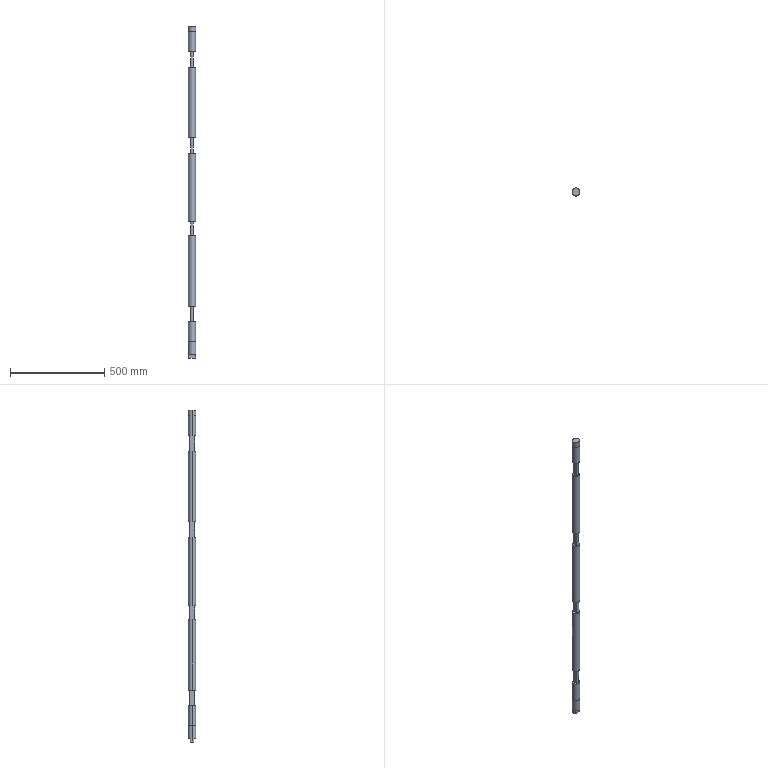Part | SolidWorks | 1 solid | 46 faces | box 40 x 40 x 1760 mm | volume 1776548 mm3 | plane 24 | cylinder 22 | commonest cylinder face diameters 38 x10 30 x8 40 x4
STEP:
#1=CARTESIAN_POINT('',(19.,0.,-258.));
#2=VERTEX_POINT('',#1);
#3=CARTESIAN_POINT('',(-19.,0.,-258.));
#4=VERTEX_POINT('',#3);
#5=CARTESIAN_POINT('',(0.,0.,-258.));
#6=DIRECTION('',(0.,0.,1.));
#7=DIRECTION('',(1.,0.,0.));
#8=AXIS2_PLACEMENT_3D('',#5,#6,#7);
#9=CIRCLE('',#8,19.);
#10=EDGE_CURVE('',#2,#4,#9,.T.);
#11=ORIENTED_EDGE('',*,*,#10,.F.);
#12=CARTESIAN_POINT('',(19.,0.,-633.5));
#13=VERTEX_POINT('',#12);
#14=CARTESIAN_POINT('',(19.,0.,-258.));
#15=DIRECTION('',(0.,0.,-1.));
#16=VECTOR('',#15,1000.);
#17=LINE('',#14,#16);
#18=EDGE_CURVE('',#2,#13,#17,.T.);
#19=ORIENTED_EDGE('',*,*,#18,.T.);
#20=CARTESIAN_POINT('',(-19.,0.,-633.5));
#21=VERTEX_POINT('',#20);
#22=CARTESIAN_POINT('',(0.,0.,-633.5));
#23=DIRECTION('',(0.,0.,1.));
#24=DIRECTION('',(1.,0.,0.));
#25=AXIS2_PLACEMENT_3D('',#22,#23,#24);
#26=CIRCLE('',#25,19.);
#27=EDGE_CURVE('',#13,#21,#26,.T.);
#28=ORIENTED_EDGE('',*,*,#27,.T.);
#29=CARTESIAN_POINT('',(-19.,0.,-258.));
#30=DIRECTION('',(0.,0.,-1.));
#31=VECTOR('',#30,1000.);
#32=LINE('',#29,#31);
#33=EDGE_CURVE('',#4,#21,#32,.T.);
#34=ORIENTED_EDGE('',*,*,#33,.F.);
#35=EDGE_LOOP('',(#11,#19,#28,#34));
#36=FACE_OUTER_BOUND('',#35,.T.);
#37=CARTESIAN_POINT('',(0.,0.,-258.));
#38=DIRECTION('',(0.,0.,-1.));
#39=DIRECTION('',(-1.,0.,0.));
#40=AXIS2_PLACEMENT_3D('',#37,#38,#39);
#41=CYLINDRICAL_SURFACE('',#40,19.);
#42=ADVANCED_FACE('',(#36),#41,.T.);
#43=CARTESIAN_POINT('',(19.,0.,-715.5));
#44=VERTEX_POINT('',#43);
#45=CARTESIAN_POINT('',(-19.,0.,-715.5));
#46=VERTEX_POINT('',#45);
#47=CARTESIAN_POINT('',(0.,0.,-715.5));
#48=DIRECTION('',(0.,0.,1.));
#49=DIRECTION('',(1.,0.,0.));
#50=AXIS2_PLACEMENT_3D('',#47,#48,#49);
#51=CIRCLE('',#50,19.);
#52=EDGE_CURVE('',#44,#46,#51,.T.);
#53=ORIENTED_EDGE('',*,*,#52,.F.);
#54=CARTESIAN_POINT('',(19.,0.,-822.5));
#55=VERTEX_POINT('',#54);
#56=CARTESIAN_POINT('',(19.,0.,-715.5));
#57=DIRECTION('',(0.,0.,-1.));
#58=VECTOR('',#57,1000.);
#59=LINE('',#56,#58);
#60=EDGE_CURVE('',#44,#55,#59,.T.);
#61=ORIENTED_EDGE('',*,*,#60,.T.);
#62=CARTESIAN_POINT('',(-19.,0.,-822.5));
#63=VERTEX_POINT('',#62);
#64=CARTESIAN_POINT('',(0.,0.,-822.5));
#65=DIRECTION('',(0.,0.,1.));
#66=DIRECTION('',(-1.,0.,0.));
#67=AXIS2_PLACEMENT_3D('',#64,#65,#66);
#68=CIRCLE('',#67,19.);
#69=EDGE_CURVE('',#55,#63,#68,.T.);
#70=ORIENTED_EDGE('',*,*,#69,.T.);
#71=CARTESIAN_POINT('',(-19.,0.,-715.5));
#72=DIRECTION('',(0.,0.,-1.));
#73=VECTOR('',#72,1000.);
#74=LINE('',#71,#73);
#75=EDGE_CURVE('',#46,#63,#74,.T.);
#76=ORIENTED_EDGE('',*,*,#75,.F.);
#77=EDGE_LOOP('',(#53,#61,#70,#76));
#78=FACE_OUTER_BOUND('',#77,.T.);
#79=CARTESIAN_POINT('',(0.,0.,-715.5));
#80=DIRECTION('',(0.,0.,-1.));
#81=DIRECTION('',(-1.,0.,0.));
#82=AXIS2_PLACEMENT_3D('',#79,#80,#81);
#83=CYLINDRICAL_SURFACE('',#82,19.);
#84=ADVANCED_FACE('',(#78),#83,.T.);
#85=CARTESIAN_POINT('',(19.,0.,-186.));
#86=VERTEX_POINT('',#85);
#87=CARTESIAN_POINT('',(-19.,0.,-186.));
#88=VERTEX_POINT('',#87);
#89=CARTESIAN_POINT('',(0.,0.,-186.));
#90=DIRECTION('',(0.,0.,1.));
#91=DIRECTION('',(1.,0.,0.));
#92=AXIS2_PLACEMENT_3D('',#89,#90,#91);
#93=CIRCLE('',#92,19.);
#94=EDGE_CURVE('',#86,#88,#93,.T.);
#95=ORIENTED_EDGE('',*,*,#94,.T.);
#96=CARTESIAN_POINT('',(-19.,0.,178.5));
#97=VERTEX_POINT('',#96);
#98=CARTESIAN_POINT('',(-19.,0.,-311.74));
#99=DIRECTION('',(0.,0.,1.));
#100=VECTOR('',#99,1000.);
#101=LINE('',#98,#100);
#102=EDGE_CURVE('',#88,#97,#101,.T.);
#103=ORIENTED_EDGE('',*,*,#102,.T.);
#104=CARTESIAN_POINT('',(19.,0.,178.5));
#105=VERTEX_POINT('',#104);
#106=CARTESIAN_POINT('',(0.,0.,178.5));
#107=DIRECTION('',(0.,0.,-1.));
#108=DIRECTION('',(-1.,0.,0.));
#109=AXIS2_PLACEMENT_3D('',#106,#107,#108);
#110=CIRCLE('',#109,19.);
#111=EDGE_CURVE('',#97,#105,#110,.T.);
#112=ORIENTED_EDGE('',*,*,#111,.T.);
#113=CARTESIAN_POINT('',(19.,0.,-311.74));
#114=DIRECTION('',(0.,0.,1.));
#115=VECTOR('',#114,1000.);
#116=LINE('',#113,#115);
#117=EDGE_CURVE('',#86,#105,#116,.T.);
#118=ORIENTED_EDGE('',*,*,#117,.F.);
#119=EDGE_LOOP('',(#95,#103,#112,#118));
#120=FACE_OUTER_BOUND('',#119,.T.);
#121=CARTESIAN_POINT('',(0.,0.,-311.74));
#122=DIRECTION('',(0.,0.,1.));
#123=DIRECTION('',(1.,0.,0.));
#124=AXIS2_PLACEMENT_3D('',#121,#122,#123);
#125=CYLINDRICAL_SURFACE('',#124,19.);
#126=ADVANCED_FACE('',(#120),#125,.T.);
#127=CARTESIAN_POINT('',(-19.,0.,715.5));
#128=VERTEX_POINT('',#127);
#129=CARTESIAN_POINT('',(19.,0.,715.5));
#130=VERTEX_POINT('',#129);
#131=CARTESIAN_POINT('',(0.,0.,715.5));
#132=DIRECTION('',(0.,0.,-1.));
#133=DIRECTION('',(-1.,0.,0.));
#134=AXIS2_PLACEMENT_3D('',#131,#132,#133);
#135=CIRCLE('',#134,19.);
#136=EDGE_CURVE('',#128,#130,#135,.T.);
#137=ORIENTED_EDGE('',*,*,#136,.F.);
#138=CARTESIAN_POINT('',(-19.,0.,822.5));
#139=VERTEX_POINT('',#138);
#140=CARTESIAN_POINT('',(-19.,0.,715.5));
#141=DIRECTION('',(0.,0.,1.));
#142=VECTOR('',#141,1000.);
#143=LINE('',#140,#142);
#144=EDGE_CURVE('',#128,#139,#143,.T.);
#145=ORIENTED_EDGE('',*,*,#144,.T.);
#146=CARTESIAN_POINT('',(19.,0.,822.5));
#147=VERTEX_POINT('',#146);
#148=CARTESIAN_POINT('',(0.,0.,822.5));
#149=DIRECTION('',(0.,0.,-1.));
#150=DIRECTION('',(1.,0.,0.));
#151=AXIS2_PLACEMENT_3D('',#148,#149,#150);
#152=CIRCLE('',#151,19.);
#153=EDGE_CURVE('',#139,#147,#152,.T.);
#154=ORIENTED_EDGE('',*,*,#153,.T.);
#155=CARTESIAN_POINT('',(19.,0.,715.5));
#156=DIRECTION('',(0.,0.,1.));
#157=VECTOR('',#156,1000.);
#158=LINE('',#155,#157);
#159=EDGE_CURVE('',#130,#147,#158,.T.);
#160=ORIENTED_EDGE('',*,*,#159,.F.);
#161=EDGE_LOOP('',(#137,#145,#154,#160));
#162=FACE_OUTER_BOUND('',#161,.T.);
#163=CARTESIAN_POINT('',(0.,0.,715.5));
#164=DIRECTION('',(0.,0.,1.));
#165=DIRECTION('',(1.,0.,0.));
#166=AXIS2_PLACEMENT_3D('',#163,#164,#165);
#167=CYLINDRICAL_SURFACE('',#166,19.);
#168=ADVANCED_FACE('',(#162),#167,.T.);
#169=CARTESIAN_POINT('',(20.,0.,852.5));
#170=VERTEX_POINT('',#169);
#171=CARTESIAN_POINT('',(-20.,0.,852.5));
#172=VERTEX_POINT('',#171);
#173=CARTESIAN_POINT('',(0.,0.,852.5));
#174=DIRECTION('',(0.,0.,1.));
#175=DIRECTION('',(1.,0.,0.));
#176=AXIS2_PLACEMENT_3D('',#173,#174,#175);
#177=CIRCLE('',#176,20.);
#178=EDGE_CURVE('',#170,#172,#177,.T.);
#179=ORIENTED_EDGE('',*,*,#178,.F.);
#180=CARTESIAN_POINT('',(20.,0.,822.5));
#181=VERTEX_POINT('',#180);
#182=CARTESIAN_POINT('',(20.,0.,852.5));
#183=DIRECTION('',(0.,0.,-1.));
#184=VECTOR('',#183,1000.);
#185=LINE('',#182,#184);
#186=EDGE_CURVE('',#170,#181,#185,.T.);
#187=ORIENTED_EDGE('',*,*,#186,.T.);
#188=CARTESIAN_POINT('',(-20.,0.,822.5));
#189=VERTEX_POINT('',#188);
#190=CARTESIAN_POINT('',(0.,0.,822.5));
#191=DIRECTION('',(0.,0.,1.));
#192=DIRECTION('',(1.,0.,0.));
#193=AXIS2_PLACEMENT_3D('',#190,#191,#192);
#194=CIRCLE('',#193,20.);
#195=EDGE_CURVE('',#181,#189,#194,.T.);
#196=ORIENTED_EDGE('',*,*,#195,.T.);
#197=CARTESIAN_POINT('',(-20.,0.,852.5));
#198=DIRECTION('',(0.,0.,-1.));
#199=VECTOR('',#198,1000.);
#200=LINE('',#197,#199);
#201=EDGE_CURVE('',#172,#189,#200,.T.);
#202=ORIENTED_EDGE('',*,*,#201,.F.);
#203=EDGE_LOOP('',(#179,#187,#196,#202));
#204=FACE_OUTER_BOUND('',#203,.T.);
#205=CARTESIAN_POINT('',(0.,0.,852.5));
#206=DIRECTION('',(0.,0.,-1.));
#207=DIRECTION('',(-1.,0.,0.));
#208=AXIS2_PLACEMENT_3D('',#205,#206,#207);
#209=CYLINDRICAL_SURFACE('',#208,20.);
#210=ADVANCED_FACE('',(#204),#209,.T.);
#211=CARTESIAN_POINT('',(-19.,0.,260.5));
#212=VERTEX_POINT('',#211);
#213=CARTESIAN_POINT('',(19.,0.,260.5));
#214=VERTEX_POINT('',#213);
#215=CARTESIAN_POINT('',(0.,0.,260.5));
#216=DIRECTION('',(0.,0.,-1.));
#217=DIRECTION('',(-1.,0.,0.));
#218=AXIS2_PLACEMENT_3D('',#215,#216,#217);
#219=CIRCLE('',#218,19.);
#220=EDGE_CURVE('',#212,#214,#219,.T.);
#221=ORIENTED_EDGE('',*,*,#220,.F.);
#222=CARTESIAN_POINT('',(-19.,0.,633.5));
#223=VERTEX_POINT('',#222);
#224=CARTESIAN_POINT('',(-19.,0.,260.5));
#225=DIRECTION('',(0.,0.,1.));
#226=VECTOR('',#225,1000.);
#227=LINE('',#224,#226);
#228=EDGE_CURVE('',#212,#223,#227,.T.);
#229=ORIENTED_EDGE('',*,*,#228,.T.);
#230=CARTESIAN_POINT('',(19.,0.,633.5));
#231=VERTEX_POINT('',#230);
#232=CARTESIAN_POINT('',(0.,0.,633.5));
#233=DIRECTION('',(0.,0.,-1.));
#234=DIRECTION('',(-1.,0.,0.));
#235=AXIS2_PLACEMENT_3D('',#232,#233,#234);
#236=CIRCLE('',#235,19.);
#237=EDGE_CURVE('',#223,#231,#236,.T.);
#238=ORIENTED_EDGE('',*,*,#237,.T.);
#239=CARTESIAN_POINT('',(19.,0.,260.5));
#240=DIRECTION('',(0.,0.,1.));
#241=VECTOR('',#240,1000.);
#242=LINE('',#239,#241);
#243=EDGE_CURVE('',#214,#231,#242,.T.);
#244=ORIENTED_EDGE('',*,*,#243,.F.);
#245=EDGE_LOOP('',(#221,#229,#238,#244));
#246=FACE_OUTER_BOUND('',#245,.T.);
#247=CARTESIAN_POINT('',(0.,0.,260.5));
#248=DIRECTION('',(0.,0.,1.));
#249=DIRECTION('',(1.,0.,0.));
#250=AXIS2_PLACEMENT_3D('',#247,#248,#249);
#251=CYLINDRICAL_SURFACE('',#250,19.);
#252=ADVANCED_FACE('',(#246),#251,.T.);
#253=CARTESIAN_POINT('',(-20.,0.,-907.5));
#254=VERTEX_POINT('',#253);
#255=CARTESIAN_POINT('',(-17.321,10.,-907.5));
#256=VERTEX_POINT('',#255);
#257=CARTESIAN_POINT('',(0.,0.,-907.5));
#258=DIRECTION('',(0.,0.,-1.));
#259=DIRECTION('',(-1.,0.,0.));
#260=AXIS2_PLACEMENT_3D('',#257,#258,#259);
#261=CIRCLE('',#260,20.);
#262=EDGE_CURVE('',#254,#256,#261,.T.);
#263=ORIENTED_EDGE('',*,*,#262,.F.);
#264=CARTESIAN_POINT('',(-20.,0.,-822.5));
#265=VERTEX_POINT('',#264);
#266=CARTESIAN_POINT('',(-20.,0.,-907.5));
#267=DIRECTION('',(0.,0.,1.));
#268=VECTOR('',#267,1000.);
#269=LINE('',#266,#268);
#270=EDGE_CURVE('',#254,#265,#269,.T.);
#271=ORIENTED_EDGE('',*,*,#270,.T.);
#272=CARTESIAN_POINT('',(20.,0.,-822.5));
#273=VERTEX_POINT('',#272);
#274=CARTESIAN_POINT('',(0.,0.,-822.5));
#275=DIRECTION('',(0.,0.,-1.));
#276=DIRECTION('',(-1.,0.,0.));
#277=AXIS2_PLACEMENT_3D('',#274,#275,#276);
#278=CIRCLE('',#277,20.);
#279=EDGE_CURVE('',#265,#273,#278,.T.);
#280=ORIENTED_EDGE('',*,*,#279,.T.);
#281=CARTESIAN_POINT('',(20.,0.,-907.5));
#282=VERTEX_POINT('',#281);
#283=CARTESIAN_POINT('',(20.,0.,-907.5));
#284=DIRECTION('',(0.,0.,1.));
#285=VECTOR('',#284,1000.);
#286=LINE('',#283,#285);
#287=EDGE_CURVE('',#282,#273,#286,.T.);
#288=ORIENTED_EDGE('',*,*,#287,.F.);
#289=CARTESIAN_POINT('',(17.321,10.,-907.5));
#290=VERTEX_POINT('',#289);
#291=CARTESIAN_POINT('',(0.,0.,-907.5));
#292=DIRECTION('',(0.,0.,-1.));
#293=DIRECTION('',(-1.,0.,0.));
#294=AXIS2_PLACEMENT_3D('',#291,#292,#293);
#295=CIRCLE('',#294,20.);
#296=EDGE_CURVE('',#290,#282,#295,.T.);
#297=ORIENTED_EDGE('',*,*,#296,.F.);
#298=CARTESIAN_POINT('',(17.321,10.,-887.5));
#299=VERTEX_POINT('',#298);
#300=CARTESIAN_POINT('',(17.321,10.,-887.5));
#301=DIRECTION('',(0.,0.,-1.));
#302=VECTOR('',#301,1000.);
#303=LINE('',#300,#302);
#304=EDGE_CURVE('',#299,#290,#303,.T.);
#305=ORIENTED_EDGE('',*,*,#304,.F.);
#306=CARTESIAN_POINT('',(-17.321,10.,-887.5));
#307=VERTEX_POINT('',#306);
#308=CARTESIAN_POINT('',(0.,0.,-887.5));
#309=DIRECTION('',(0.,0.,-1.));
#310=DIRECTION('',(-1.,0.,0.));
#311=AXIS2_PLACEMENT_3D('',#308,#309,#310);
#312=CIRCLE('',#311,20.);
#313=EDGE_CURVE('',#307,#299,#312,.T.);
#314=ORIENTED_EDGE('',*,*,#313,.F.);
#315=CARTESIAN_POINT('',(-17.321,10.,-887.5));
#316=DIRECTION('',(0.,0.,-1.));
#317=VECTOR('',#316,1000.);
#318=LINE('',#315,#317);
#319=EDGE_CURVE('',#307,#256,#318,.T.);
#320=ORIENTED_EDGE('',*,*,#319,.T.);
#321=EDGE_LOOP('',(#263,#271,#280,#288,#297,#305,#314,#320));
#322=FACE_OUTER_BOUND('',#321,.T.);
#323=CARTESIAN_POINT('',(0.,0.,-907.5));
#324=DIRECTION('',(0.,0.,1.));
#325=DIRECTION('',(1.,0.,0.));
#326=AXIS2_PLACEMENT_3D('',#323,#324,#325);
#327=CYLINDRICAL_SURFACE('',#326,20.);
#328=ADVANCED_FACE('',(#322),#327,.T.);
#329=CARTESIAN_POINT('',(-17.321,-10.,-907.5));
#330=VERTEX_POINT('',#329);
#331=CARTESIAN_POINT('',(0.,0.,-907.5));
#332=DIRECTION('',(0.,0.,-1.));
#333=DIRECTION('',(-1.,0.,0.));
#334=AXIS2_PLACEMENT_3D('',#331,#332,#333);
#335=CIRCLE('',#334,20.);
#336=EDGE_CURVE('',#330,#254,#335,.T.);
#337=ORIENTED_EDGE('',*,*,#336,.T.);
#338=ORIENTED_EDGE('',*,*,#262,.T.);
#339=CARTESIAN_POINT('',(0.,10.,-907.5));
#340=DIRECTION('',(1.,0.,0.));
#341=VECTOR('',#340,1000.);
#342=LINE('',#339,#341);
#343=EDGE_CURVE('',#256,#290,#342,.T.);
#344=ORIENTED_EDGE('',*,*,#343,.T.);
#345=ORIENTED_EDGE('',*,*,#296,.T.);
#346=CARTESIAN_POINT('',(17.321,-10.,-907.5));
#347=VERTEX_POINT('',#346);
#348=CARTESIAN_POINT('',(0.,0.,-907.5));
#349=DIRECTION('',(0.,0.,-1.));
#350=DIRECTION('',(-1.,0.,0.));
#351=AXIS2_PLACEMENT_3D('',#348,#349,#350);
#352=CIRCLE('',#351,20.);
#353=EDGE_CURVE('',#282,#347,#352,.T.);
#354=ORIENTED_EDGE('',*,*,#353,.T.);
#355=CARTESIAN_POINT('',(0.,-10.,-907.5));
#356=DIRECTION('',(1.,0.,0.));
#357=VECTOR('',#356,1000.);
#358=LINE('',#355,#357);
#359=EDGE_CURVE('',#330,#347,#358,.T.);
#360=ORIENTED_EDGE('',*,*,#359,.F.);
#361=EDGE_LOOP('',(#337,#338,#344,#345,#354,#360));
#362=FACE_OUTER_BOUND('',#361,.T.);
#363=CARTESIAN_POINT('',(0.,0.,-907.5));
#364=DIRECTION('',(0.,0.,-1.));
#365=DIRECTION('',(-1.,0.,0.));
#366=AXIS2_PLACEMENT_3D('',#363,#364,#365);
#367=PLANE('',#366);
#368=ADVANCED_FACE('',(#362),#367,.T.);
#369=ORIENTED_EDGE('',*,*,#270,.F.);
#370=ORIENTED_EDGE('',*,*,#336,.F.);
#371=CARTESIAN_POINT('',(-17.321,-10.,-887.5));
#372=VERTEX_POINT('',#371);
#373=CARTESIAN_POINT('',(-17.321,-10.,-887.5));
#374=DIRECTION('',(0.,0.,-1.));
#375=VECTOR('',#374,1000.);
#376=LINE('',#373,#375);
#377=EDGE_CURVE('',#372,#330,#376,.T.);
#378=ORIENTED_EDGE('',*,*,#377,.F.);
#379=CARTESIAN_POINT('',(17.321,-10.,-887.5));
#380=VERTEX_POINT('',#379);
#381=CARTESIAN_POINT('',(0.,0.,-887.5));
#382=DIRECTION('',(0.,0.,-1.));
#383=DIRECTION('',(-1.,0.,0.));
#384=AXIS2_PLACEMENT_3D('',#381,#382,#383);
#385=CIRCLE('',#384,20.);
#386=EDGE_CURVE('',#380,#372,#385,.T.);
#387=ORIENTED_EDGE('',*,*,#386,.F.);
#388=CARTESIAN_POINT('',(17.321,-10.,-887.5));
#389=DIRECTION('',(0.,0.,-1.));
#390=VECTOR('',#389,1000.);
#391=LINE('',#388,#390);
#392=EDGE_CURVE('',#380,#347,#391,.T.);
#393=ORIENTED_EDGE('',*,*,#392,.T.);
#394=ORIENTED_EDGE('',*,*,#353,.F.);
#395=ORIENTED_EDGE('',*,*,#287,.T.);
#396=CARTESIAN_POINT('',(0.,0.,-822.5));
#397=DIRECTION('',(0.,0.,-1.));
#398=DIRECTION('',(-1.,0.,0.));
#399=AXIS2_PLACEMENT_3D('',#396,#397,#398);
#400=CIRCLE('',#399,20.);
#401=EDGE_CURVE('',#273,#265,#400,.T.);
#402=ORIENTED_EDGE('',*,*,#401,.T.);
#403=EDGE_LOOP('',(#369,#370,#378,#387,#393,#394,#395,#402));
#404=FACE_OUTER_BOUND('',#403,.T.);
#405=CARTESIAN_POINT('',(0.,0.,-907.5));
#406=DIRECTION('',(0.,0.,1.));
#407=DIRECTION('',(1.,0.,0.));
#408=AXIS2_PLACEMENT_3D('',#405,#406,#407);
#409=CYLINDRICAL_SURFACE('',#408,20.);
#410=ADVANCED_FACE('',(#404),#409,.T.);
#411=CARTESIAN_POINT('',(7.5,-12.99,260.5));
#412=VERTEX_POINT('',#411);
#413=CARTESIAN_POINT('',(7.5,-12.99,178.5));
#414=VERTEX_POINT('',#413);
#415=CARTESIAN_POINT('',(7.5,-12.99,822.5));
#416=DIRECTION('',(0.,0.,-1.));
#417=VECTOR('',#416,1000.);
#418=LINE('',#415,#417);
#419=EDGE_CURVE('',#412,#414,#418,.T.);
#420=ORIENTED_EDGE('',*,*,#419,.T.);
#421=CARTESIAN_POINT('',(7.5,12.99,178.5));
#422=VERTEX_POINT('',#421);
#423=CARTESIAN_POINT('',(7.5,0.,178.5));
#424=DIRECTION('',(0.,1.,0.));
#425=VECTOR('',#424,1000.);
#426=LINE('',#423,#425);
#427=EDGE_CURVE('',#414,#422,#426,.T.);
#428=ORIENTED_EDGE('',*,*,#427,.T.);
#429=CARTESIAN_POINT('',(7.5,12.99,260.5));
#430=VERTEX_POINT('',#429);
#431=CARTESIAN_POINT('',(7.5,12.99,822.5));
#432=DIRECTION('',(0.,0.,-1.));
#433=VECTOR('',#432,1000.);
#434=LINE('',#431,#433);
#435=EDGE_CURVE('',#430,#422,#434,.T.);
#436=ORIENTED_EDGE('',*,*,#435,.F.);
#437=CARTESIAN_POINT('',(7.5,0.,260.5));
#438=DIRECTION('',(0.,1.,0.));
#439=VECTOR('',#438,1000.);
#440=LINE('',#437,#439);
#441=EDGE_CURVE('',#412,#430,#440,.T.);
#442=ORIENTED_EDGE('',*,*,#441,.F.);
#443=EDGE_LOOP('',(#420,#428,#436,#442));
#444=FACE_OUTER_BOUND('',#443,.T.);
#445=CARTESIAN_POINT('',(7.5,0.,822.5));
#446=DIRECTION('',(1.,0.,0.));
#447=DIRECTION('',(0.,0.,-1.));
#448=AXIS2_PLACEMENT_3D('',#445,#446,#447);
#449=PLANE('',#448);
#450=ADVANCED_FACE('',(#444),#449,.T.);
#451=CARTESIAN_POINT('',(-7.5,-12.99,178.5));
#452=VERTEX_POINT('',#451);
#453=CARTESIAN_POINT('',(0.,0.,178.5));
#454=DIRECTION('',(0.,0.,-1.));
#455=DIRECTION('',(-1.,0.,0.));
#456=AXIS2_PLACEMENT_3D('',#453,#454,#455);
#457=CIRCLE('',#456,15.);
#458=EDGE_CURVE('',#414,#452,#457,.T.);
#459=ORIENTED_EDGE('',*,*,#458,.F.);
#460=ORIENTED_EDGE('',*,*,#419,.F.);
#461=CARTESIAN_POINT('',(-7.5,-12.99,260.5));
#462=VERTEX_POINT('',#461);
#463=CARTESIAN_POINT('',(0.,0.,260.5));
#464=DIRECTION('',(0.,0.,-1.));
#465=DIRECTION('',(-1.,0.,0.));
#466=AXIS2_PLACEMENT_3D('',#463,#464,#465);
#467=CIRCLE('',#466,15.);
#468=EDGE_CURVE('',#412,#462,#467,.T.);
#469=ORIENTED_EDGE('',*,*,#468,.T.);
#470=CARTESIAN_POINT('',(-7.5,-12.99,822.5));
#471=DIRECTION('',(0.,0.,-1.));
#472=VECTOR('',#471,1000.);
#473=LINE('',#470,#472);
#474=EDGE_CURVE('',#462,#452,#473,.T.);
#475=ORIENTED_EDGE('',*,*,#474,.T.);
#476=EDGE_LOOP('',(#459,#460,#469,#475));
#477=FACE_OUTER_BOUND('',#476,.T.);
#478=CARTESIAN_POINT('',(0.,0.,822.5));
#479=DIRECTION('',(0.,0.,-1.));
#480=DIRECTION('',(-1.,0.,0.));
#481=AXIS2_PLACEMENT_3D('',#478,#479,#480);
#482=CYLINDRICAL_SURFACE('',#481,15.);
#483=ADVANCED_FACE('',(#477),#482,.T.);
#484=CARTESIAN_POINT('',(-7.5,12.99,178.5));
#485=VERTEX_POINT('',#484);
#486=CARTESIAN_POINT('',(-7.5,0.,178.5));
#487=DIRECTION('',(0.,1.,0.));
#488=VECTOR('',#487,1000.);
#489=LINE('',#486,#488);
#490=EDGE_CURVE('',#452,#485,#489,.T.);
#491=ORIENTED_EDGE('',*,*,#490,.F.);
#492=ORIENTED_EDGE('',*,*,#474,.F.);
#493=CARTESIAN_POINT('',(-7.5,12.99,260.5));
#494=VERTEX_POINT('',#493);
#495=CARTESIAN_POINT('',(-7.5,0.,260.5));
#496=DIRECTION('',(0.,1.,0.));
#497=VECTOR('',#496,1000.);
#498=LINE('',#495,#497);
#499=EDGE_CURVE('',#462,#494,#498,.T.);
#500=ORIENTED_EDGE('',*,*,#499,.T.);
#501=CARTESIAN_POINT('',(-7.5,12.99,822.5));
#502=DIRECTION('',(0.,0.,-1.));
#503=VECTOR('',#502,1000.);
#504=LINE('',#501,#503);
#505=EDGE_CURVE('',#494,#485,#504,.T.);
#506=ORIENTED_EDGE('',*,*,#505,.T.);
#507=EDGE_LOOP('',(#491,#492,#500,#506));
#508=FACE_OUTER_BOUND('',#507,.T.);
#509=CARTESIAN_POINT('',(-7.5,0.,822.5));
#510=DIRECTION('',(1.,0.,0.));
#511=DIRECTION('',(0.,0.,-1.));
#512=AXIS2_PLACEMENT_3D('',#509,#510,#511);
#513=PLANE('',#512);
#514=ADVANCED_FACE('',(#508),#513,.F.);
#515=CARTESIAN_POINT('',(0.,0.,178.5));
#516=DIRECTION('',(0.,0.,-1.));
#517=DIRECTION('',(-1.,0.,0.));
#518=AXIS2_PLACEMENT_3D('',#515,#516,#517);
#519=CIRCLE('',#518,15.);
#520=EDGE_CURVE('',#485,#422,#519,.T.);
#521=ORIENTED_EDGE('',*,*,#520,.F.);
#522=ORIENTED_EDGE('',*,*,#505,.F.);
#523=CARTESIAN_POINT('',(0.,0.,260.5));
#524=DIRECTION('',(0.,0.,-1.));
#525=DIRECTION('',(-1.,0.,0.));
#526=AXIS2_PLACEMENT_3D('',#523,#524,#525);
#527=CIRCLE('',#526,15.);
#528=EDGE_CURVE('',#494,#430,#527,.T.);
#529=ORIENTED_EDGE('',*,*,#528,.T.);
#530=ORIENTED_EDGE('',*,*,#435,.T.);
#531=EDGE_LOOP('',(#521,#522,#529,#530));
#532=FACE_OUTER_BOUND('',#531,.T.);
#533=CARTESIAN_POINT('',(0.,0.,822.5));
#534=DIRECTION('',(0.,0.,-1.));
#535=DIRECTION('',(-1.,0.,0.));
#536=AXIS2_PLACEMENT_3D('',#533,#534,#535);
#537=CYLINDRICAL_SURFACE('',#536,15.);
#538=ADVANCED_FACE('',(#532),#537,.T.);
#539=CARTESIAN_POINT('',(0.,0.,260.5));
#540=DIRECTION('',(0.,0.,-1.));
#541=DIRECTION('',(-1.,0.,0.));
#542=AXIS2_PLACEMENT_3D('',#539,#540,#541);
#543=CIRCLE('',#542,19.);
#544=EDGE_CURVE('',#214,#212,#543,.T.);
#545=ORIENTED_EDGE('',*,*,#544,.T.);
#546=ORIENTED_EDGE('',*,*,#220,.T.);
#547=EDGE_LOOP('',(#545,#546));
#548=FACE_OUTER_BOUND('',#547,.T.);
#549=ORIENTED_EDGE('',*,*,#468,.F.);
#550=ORIENTED_EDGE('',*,*,#441,.T.);
#551=ORIENTED_EDGE('',*,*,#528,.F.);
#552=ORIENTED_EDGE('',*,*,#499,.F.);
#553=EDGE_LOOP('',(#549,#550,#551,#552));
#554=FACE_BOUND('',#553,.T.);
#555=CARTESIAN_POINT('',(0.,0.,260.5));
#556=DIRECTION('',(0.,0.,-1.));
#557=DIRECTION('',(-1.,0.,0.));
#558=AXIS2_PLACEMENT_3D('',#555,#556,#557);
#559=PLANE('',#558);
#560=ADVANCED_FACE('',(#548,#554),#559,.T.);
#561=CARTESIAN_POINT('',(0.,0.,633.5));
#562=DIRECTION('',(0.,0.,-1.));
#563=DIRECTION('',(-1.,0.,0.));
#564=AXIS2_PLACEMENT_3D('',#561,#562,#563);
#565=CIRCLE('',#564,19.);
#566=EDGE_CURVE('',#231,#223,#565,.T.);
#567=ORIENTED_EDGE('',*,*,#566,.F.);
#568=ORIENTED_EDGE('',*,*,#237,.F.);
#569=EDGE_LOOP('',(#567,#568));
#570=FACE_OUTER_BOUND('',#569,.T.);
#571=CARTESIAN_POINT('',(7.5,-12.99,633.5));
#572=VERTEX_POINT('',#571);
#573=CARTESIAN_POINT('',(7.5,12.99,633.5));
#574=VERTEX_POINT('',#573);
#575=CARTESIAN_POINT('',(7.5,0.,633.5));
#576=DIRECTION('',(0.,1.,0.));
#577=VECTOR('',#576,1000.);
#578=LINE('',#575,#577);
#579=EDGE_CURVE('',#572,#574,#578,.T.);
#580=ORIENTED_EDGE('',*,*,#579,.F.);
#581=CARTESIAN_POINT('',(-7.5,-12.99,633.5));
#582=VERTEX_POINT('',#581);
#583=CARTESIAN_POINT('',(0.,0.,633.5));
#584=DIRECTION('',(0.,0.,-1.));
#585=DIRECTION('',(-1.,0.,0.));
#586=AXIS2_PLACEMENT_3D('',#583,#584,#585);
#587=CIRCLE('',#586,15.);
#588=EDGE_CURVE('',#572,#582,#587,.T.);
#589=ORIENTED_EDGE('',*,*,#588,.T.);
#590=CARTESIAN_POINT('',(-7.5,12.99,633.5));
#591=VERTEX_POINT('',#590);
#592=CARTESIAN_POINT('',(-7.5,0.,633.5));
#593=DIRECTION('',(0.,1.,0.));
#594=VECTOR('',#593,1000.);
#595=LINE('',#592,#594);
#596=EDGE_CURVE('',#582,#591,#595,.T.);
#597=ORIENTED_EDGE('',*,*,#596,.T.);
#598=CARTESIAN_POINT('',(0.,0.,633.5));
#599=DIRECTION('',(0.,0.,-1.));
#600=DIRECTION('',(-1.,0.,0.));
#601=AXIS2_PLACEMENT_3D('',#598,#599,#600);
#602=CIRCLE('',#601,15.);
#603=EDGE_CURVE('',#591,#574,#602,.T.);
#604=ORIENTED_EDGE('',*,*,#603,.T.);
#605=EDGE_LOOP('',(#580,#589,#597,#604));
#606=FACE_BOUND('',#605,.T.);
#607=CARTESIAN_POINT('',(0.,0.,633.5));
#608=DIRECTION('',(0.,0.,-1.));
#609=DIRECTION('',(-1.,0.,0.));
#610=AXIS2_PLACEMENT_3D('',#607,#608,#609);
#611=PLANE('',#610);
#612=ADVANCED_FACE('',(#570,#606),#611,.F.);
#613=ORIENTED_EDGE('',*,*,#228,.F.);
#614=ORIENTED_EDGE('',*,*,#544,.F.);
#615=ORIENTED_EDGE('',*,*,#243,.T.);
#616=ORIENTED_EDGE('',*,*,#566,.T.);
#617=EDGE_LOOP('',(#613,#614,#615,#616));
#618=FACE_OUTER_BOUND('',#617,.T.);
#619=CARTESIAN_POINT('',(0.,0.,260.5));
#620=DIRECTION('',(0.,0.,1.));
#621=DIRECTION('',(1.,0.,0.));
#622=AXIS2_PLACEMENT_3D('',#619,#620,#621);
#623=CYLINDRICAL_SURFACE('',#622,19.);
#624=ADVANCED_FACE('',(#618),#623,.T.);
#625=CARTESIAN_POINT('',(0.,0.,852.5));
#626=DIRECTION('',(0.,0.,1.));
#627=DIRECTION('',(1.,0.,0.));
#628=AXIS2_PLACEMENT_3D('',#625,#626,#627);
#629=CIRCLE('',#628,20.);
#630=EDGE_CURVE('',#172,#170,#629,.T.);
#631=ORIENTED_EDGE('',*,*,#630,.T.);
#632=ORIENTED_EDGE('',*,*,#178,.T.);
#633=EDGE_LOOP('',(#631,#632));
#634=FACE_OUTER_BOUND('',#633,.T.);
#635=CARTESIAN_POINT('',(0.,0.,852.5));
#636=DIRECTION('',(0.,0.,1.));
#637=DIRECTION('',(1.,0.,0.));
#638=AXIS2_PLACEMENT_3D('',#635,#636,#637);
#639=PLANE('',#638);
#640=ADVANCED_FACE('',(#634),#639,.T.);
#641=ORIENTED_EDGE('',*,*,#186,.F.);
#642=ORIENTED_EDGE('',*,*,#630,.F.);
#643=ORIENTED_EDGE('',*,*,#201,.T.);
#644=CARTESIAN_POINT('',(0.,0.,822.5));
#645=DIRECTION('',(0.,0.,1.));
#646=DIRECTION('',(1.,0.,0.));
#647=AXIS2_PLACEMENT_3D('',#644,#645,#646);
#648=CIRCLE('',#647,20.);
#649=EDGE_CURVE('',#189,#181,#648,.T.);
#650=ORIENTED_EDGE('',*,*,#649,.T.);
#651=EDGE_LOOP('',(#641,#642,#643,#650));
#652=FACE_OUTER_BOUND('',#651,.T.);
#653=CARTESIAN_POINT('',(0.,0.,852.5));
#654=DIRECTION('',(0.,0.,-1.));
#655=DIRECTION('',(-1.,0.,0.));
#656=AXIS2_PLACEMENT_3D('',#653,#654,#655);
#657=CYLINDRICAL_SURFACE('',#656,20.);
#658=ADVANCED_FACE('',(#652),#657,.T.);
#659=CARTESIAN_POINT('',(0.,0.,822.5));
#660=DIRECTION('',(0.,0.,-1.));
#661=DIRECTION('',(1.,0.,0.));
#662=AXIS2_PLACEMENT_3D('',#659,#660,#661);
#663=CIRCLE('',#662,19.);
#664=EDGE_CURVE('',#147,#139,#663,.T.);
#665=ORIENTED_EDGE('',*,*,#664,.F.);
#666=ORIENTED_EDGE('',*,*,#153,.F.);
#667=EDGE_LOOP('',(#665,#666));
#668=FACE_BOUND('',#667,.T.);
#669=ORIENTED_EDGE('',*,*,#649,.F.);
#670=ORIENTED_EDGE('',*,*,#195,.F.);
#671=EDGE_LOOP('',(#669,#670));
#672=FACE_OUTER_BOUND('',#671,.T.);
#673=CARTESIAN_POINT('',(0.,0.,822.5));
#674=DIRECTION('',(0.,0.,1.));
#675=DIRECTION('',(1.,0.,0.));
#676=AXIS2_PLACEMENT_3D('',#673,#674,#675);
#677=PLANE('',#676);
#678=ADVANCED_FACE('',(#668,#672),#677,.F.);
#679=ORIENTED_EDGE('',*,*,#144,.F.);
#680=CARTESIAN_POINT('',(0.,0.,715.5));
#681=DIRECTION('',(0.,0.,-1.));
#682=DIRECTION('',(-1.,0.,0.));
#683=AXIS2_PLACEMENT_3D('',#680,#681,#682);
#684=CIRCLE('',#683,19.);
#685=EDGE_CURVE('',#130,#128,#684,.T.);
#686=ORIENTED_EDGE('',*,*,#685,.F.);
#687=ORIENTED_EDGE('',*,*,#159,.T.);
#688=ORIENTED_EDGE('',*,*,#664,.T.);
#689=EDGE_LOOP('',(#679,#686,#687,#688));
#690=FACE_OUTER_BOUND('',#689,.T.);
#691=CARTESIAN_POINT('',(0.,0.,715.5));
#692=DIRECTION('',(0.,0.,1.));
#693=DIRECTION('',(1.,0.,0.));
#694=AXIS2_PLACEMENT_3D('',#691,#692,#693);
#695=CYLINDRICAL_SURFACE('',#694,19.);
#696=ADVANCED_FACE('',(#690),#695,.T.);
#697=ORIENTED_EDGE('',*,*,#685,.T.);
#698=ORIENTED_EDGE('',*,*,#136,.T.);
#699=EDGE_LOOP('',(#697,#698));
#700=FACE_OUTER_BOUND('',#699,.T.);
#701=CARTESIAN_POINT('',(7.5,-12.99,715.5));
#702=VERTEX_POINT('',#701);
#703=CARTESIAN_POINT('',(-7.5,-12.99,715.5));
#704=VERTEX_POINT('',#703);
#705=CARTESIAN_POINT('',(0.,0.,715.5));
#706=DIRECTION('',(0.,0.,-1.));
#707=DIRECTION('',(-1.,0.,0.));
#708=AXIS2_PLACEMENT_3D('',#705,#706,#707);
#709=CIRCLE('',#708,15.);
#710=EDGE_CURVE('',#702,#704,#709,.T.);
#711=ORIENTED_EDGE('',*,*,#710,.F.);
#712=CARTESIAN_POINT('',(7.5,12.99,715.5));
#713=VERTEX_POINT('',#712);
#714=CARTESIAN_POINT('',(7.5,0.,715.5));
#715=DIRECTION('',(0.,1.,0.));
#716=VECTOR('',#715,1000.);
#717=LINE('',#714,#716);
#718=EDGE_CURVE('',#702,#713,#717,.T.);
#719=ORIENTED_EDGE('',*,*,#718,.T.);
#720=CARTESIAN_POINT('',(-7.5,12.99,715.5));
#721=VERTEX_POINT('',#720);
#722=CARTESIAN_POINT('',(0.,0.,715.5));
#723=DIRECTION('',(0.,0.,-1.));
#724=DIRECTION('',(-1.,0.,0.));
#725=AXIS2_PLACEMENT_3D('',#722,#723,#724);
#726=CIRCLE('',#725,15.);
#727=EDGE_CURVE('',#721,#713,#726,.T.);
#728=ORIENTED_EDGE('',*,*,#727,.F.);
#729=CARTESIAN_POINT('',(-7.5,0.,715.5));
#730=DIRECTION('',(0.,1.,0.));
#731=VECTOR('',#730,1000.);
#732=LINE('',#729,#731);
#733=EDGE_CURVE('',#704,#721,#732,.T.);
#734=ORIENTED_EDGE('',*,*,#733,.F.);
#735=EDGE_LOOP('',(#711,#719,#728,#734));
#736=FACE_BOUND('',#735,.T.);
#737=CARTESIAN_POINT('',(0.,0.,715.5));
#738=DIRECTION('',(0.,0.,-1.));
#739=DIRECTION('',(-1.,0.,0.));
#740=AXIS2_PLACEMENT_3D('',#737,#738,#739);
#741=PLANE('',#740);
#742=ADVANCED_FACE('',(#700,#736),#741,.T.);
#743=ORIENTED_EDGE('',*,*,#603,.F.);
#744=CARTESIAN_POINT('',(-7.5,12.99,822.5));
#745=DIRECTION('',(0.,0.,-1.));
#746=VECTOR('',#745,1000.);
#747=LINE('',#744,#746);
#748=EDGE_CURVE('',#721,#591,#747,.T.);
#749=ORIENTED_EDGE('',*,*,#748,.F.);
#750=ORIENTED_EDGE('',*,*,#727,.T.);
#751=CARTESIAN_POINT('',(7.5,12.99,822.5));
#752=DIRECTION('',(0.,0.,-1.));
#753=VECTOR('',#752,1000.);
#754=LINE('',#751,#753);
#755=EDGE_CURVE('',#713,#574,#754,.T.);
#756=ORIENTED_EDGE('',*,*,#755,.T.);
#757=EDGE_LOOP('',(#743,#749,#750,#756));
#758=FACE_OUTER_BOUND('',#757,.T.);
#759=CARTESIAN_POINT('',(0.,0.,822.5));
#760=DIRECTION('',(0.,0.,-1.));
#761=DIRECTION('',(-1.,0.,0.));
#762=AXIS2_PLACEMENT_3D('',#759,#760,#761);
#763=CYLINDRICAL_SURFACE('',#762,15.);
#764=ADVANCED_FACE('',(#758),#763,.T.);
#765=ORIENTED_EDGE('',*,*,#596,.F.);
#766=CARTESIAN_POINT('',(-7.5,-12.99,822.5));
#767=DIRECTION('',(0.,0.,-1.));
#768=VECTOR('',#767,1000.);
#769=LINE('',#766,#768);
#770=EDGE_CURVE('',#704,#582,#769,.T.);
#771=ORIENTED_EDGE('',*,*,#770,.F.);
#772=ORIENTED_EDGE('',*,*,#733,.T.);
#773=ORIENTED_EDGE('',*,*,#748,.T.);
#774=EDGE_LOOP('',(#765,#771,#772,#773));
#775=FACE_OUTER_BOUND('',#774,.T.);
#776=CARTESIAN_POINT('',(-7.5,0.,822.5));
#777=DIRECTION('',(1.,0.,0.));
#778=DIRECTION('',(0.,0.,-1.));
#779=AXIS2_PLACEMENT_3D('',#776,#777,#778);
#780=PLANE('',#779);
#781=ADVANCED_FACE('',(#775),#780,.F.);
#782=ORIENTED_EDGE('',*,*,#588,.F.);
#783=CARTESIAN_POINT('',(7.5,-12.99,822.5));
#784=DIRECTION('',(0.,0.,-1.));
#785=VECTOR('',#784,1000.);
#786=LINE('',#783,#785);
#787=EDGE_CURVE('',#702,#572,#786,.T.);
#788=ORIENTED_EDGE('',*,*,#787,.F.);
#789=ORIENTED_EDGE('',*,*,#710,.T.);
#790=ORIENTED_EDGE('',*,*,#770,.T.);
#791=EDGE_LOOP('',(#782,#788,#789,#790));
#792=FACE_OUTER_BOUND('',#791,.T.);
#793=CARTESIAN_POINT('',(0.,0.,822.5));
#794=DIRECTION('',(0.,0.,-1.));
#795=DIRECTION('',(-1.,0.,0.));
#796=AXIS2_PLACEMENT_3D('',#793,#794,#795);
#797=CYLINDRICAL_SURFACE('',#796,15.);
#798=ADVANCED_FACE('',(#792),#797,.T.);
#799=ORIENTED_EDGE('',*,*,#787,.T.);
#800=ORIENTED_EDGE('',*,*,#579,.T.);
#801=ORIENTED_EDGE('',*,*,#755,.F.);
#802=ORIENTED_EDGE('',*,*,#718,.F.);
#803=EDGE_LOOP('',(#799,#800,#801,#802));
#804=FACE_OUTER_BOUND('',#803,.T.);
#805=CARTESIAN_POINT('',(7.5,0.,822.5));
#806=DIRECTION('',(1.,0.,0.));
#807=DIRECTION('',(0.,0.,-1.));
#808=AXIS2_PLACEMENT_3D('',#805,#806,#807);
#809=PLANE('',#808);
#810=ADVANCED_FACE('',(#804),#809,.T.);
#811=CARTESIAN_POINT('',(0.,0.,178.5));
#812=DIRECTION('',(0.,0.,-1.));
#813=DIRECTION('',(-1.,0.,0.));
#814=AXIS2_PLACEMENT_3D('',#811,#812,#813);
#815=CIRCLE('',#814,19.);
#816=EDGE_CURVE('',#105,#97,#815,.T.);
#817=ORIENTED_EDGE('',*,*,#816,.F.);
#818=ORIENTED_EDGE('',*,*,#111,.F.);
#819=EDGE_LOOP('',(#817,#818));
#820=FACE_OUTER_BOUND('',#819,.T.);
#821=ORIENTED_EDGE('',*,*,#427,.F.);
#822=ORIENTED_EDGE('',*,*,#458,.T.);
#823=ORIENTED_EDGE('',*,*,#490,.T.);
#824=ORIENTED_EDGE('',*,*,#520,.T.);
#825=EDGE_LOOP('',(#821,#822,#823,#824));
#826=FACE_BOUND('',#825,.T.);
#827=CARTESIAN_POINT('',(0.,0.,178.5));
#828=DIRECTION('',(0.,0.,-1.));
#829=DIRECTION('',(-1.,0.,0.));
#830=AXIS2_PLACEMENT_3D('',#827,#828,#829);
#831=PLANE('',#830);
#832=ADVANCED_FACE('',(#820,#826),#831,.F.);
#833=ORIENTED_EDGE('',*,*,#94,.F.);
#834=CARTESIAN_POINT('',(0.,0.,-186.));
#835=DIRECTION('',(0.,0.,1.));
#836=DIRECTION('',(1.,0.,0.));
#837=AXIS2_PLACEMENT_3D('',#834,#835,#836);
#838=CIRCLE('',#837,19.);
#839=EDGE_CURVE('',#88,#86,#838,.T.);
#840=ORIENTED_EDGE('',*,*,#839,.F.);
#841=EDGE_LOOP('',(#833,#840));
#842=FACE_OUTER_BOUND('',#841,.T.);
#843=CARTESIAN_POINT('',(7.5,12.99,-186.));
#844=VERTEX_POINT('',#843);
#845=CARTESIAN_POINT('',(7.5,-12.99,-186.));
#846=VERTEX_POINT('',#845);
#847=CARTESIAN_POINT('',(7.5,0.,-186.));
#848=DIRECTION('',(0.,-1.,0.));
#849=VECTOR('',#848,1000.);
#850=LINE('',#847,#849);
#851=EDGE_CURVE('',#844,#846,#850,.T.);
#852=ORIENTED_EDGE('',*,*,#851,.F.);
#853=CARTESIAN_POINT('',(-7.5,12.99,-186.));
#854=VERTEX_POINT('',#853);
#855=CARTESIAN_POINT('',(0.,0.,-186.));
#856=DIRECTION('',(0.,0.,1.));
#857=DIRECTION('',(1.,0.,0.));
#858=AXIS2_PLACEMENT_3D('',#855,#856,#857);
#859=CIRCLE('',#858,15.);
#860=EDGE_CURVE('',#844,#854,#859,.T.);
#861=ORIENTED_EDGE('',*,*,#860,.T.);
#862=CARTESIAN_POINT('',(-7.5,-12.99,-186.));
#863=VERTEX_POINT('',#862);
#864=CARTESIAN_POINT('',(-7.5,0.,-186.));
#865=DIRECTION('',(0.,-1.,0.));
#866=VECTOR('',#865,1000.);
#867=LINE('',#864,#866);
#868=EDGE_CURVE('',#854,#863,#867,.T.);
#869=ORIENTED_EDGE('',*,*,#868,.T.);
#870=CARTESIAN_POINT('',(0.,0.,-186.));
#871=DIRECTION('',(0.,0.,1.));
#872=DIRECTION('',(1.,0.,0.));
#873=AXIS2_PLACEMENT_3D('',#870,#871,#872);
#874=CIRCLE('',#873,15.);
#875=EDGE_CURVE('',#863,#846,#874,.T.);
#876=ORIENTED_EDGE('',*,*,#875,.T.);
#877=EDGE_LOOP('',(#852,#861,#869,#876));
#878=FACE_BOUND('',#877,.T.);
#879=CARTESIAN_POINT('',(0.,0.,-186.));
#880=DIRECTION('',(0.,0.,1.));
#881=DIRECTION('',(1.,0.,0.));
#882=AXIS2_PLACEMENT_3D('',#879,#880,#881);
#883=PLANE('',#882);
#884=ADVANCED_FACE('',(#842,#878),#883,.F.);
#885=ORIENTED_EDGE('',*,*,#102,.F.);
#886=ORIENTED_EDGE('',*,*,#839,.T.);
#887=ORIENTED_EDGE('',*,*,#117,.T.);
#888=ORIENTED_EDGE('',*,*,#816,.T.);
#889=EDGE_LOOP('',(#885,#886,#887,#888));
#890=FACE_OUTER_BOUND('',#889,.T.);
#891=CARTESIAN_POINT('',(0.,0.,-311.74));
#892=DIRECTION('',(0.,0.,1.));
#893=DIRECTION('',(1.,0.,0.));
#894=AXIS2_PLACEMENT_3D('',#891,#892,#893);
#895=CYLINDRICAL_SURFACE('',#894,19.);
#896=ADVANCED_FACE('',(#890),#895,.T.);
#897=CARTESIAN_POINT('',(0.,0.,-822.5));
#898=DIRECTION('',(0.,0.,1.));
#899=DIRECTION('',(-1.,0.,0.));
#900=AXIS2_PLACEMENT_3D('',#897,#898,#899);
#901=CIRCLE('',#900,19.);
#902=EDGE_CURVE('',#63,#55,#901,.T.);
#903=ORIENTED_EDGE('',*,*,#902,.F.);
#904=ORIENTED_EDGE('',*,*,#69,.F.);
#905=EDGE_LOOP('',(#903,#904));
#906=FACE_BOUND('',#905,.T.);
#907=ORIENTED_EDGE('',*,*,#401,.F.);
#908=ORIENTED_EDGE('',*,*,#279,.F.);
#909=EDGE_LOOP('',(#907,#908));
#910=FACE_OUTER_BOUND('',#909,.T.);
#911=CARTESIAN_POINT('',(0.,0.,-822.5));
#912=DIRECTION('',(0.,0.,-1.));
#913=DIRECTION('',(-1.,0.,0.));
#914=AXIS2_PLACEMENT_3D('',#911,#912,#913);
#915=PLANE('',#914);
#916=ADVANCED_FACE('',(#906,#910),#915,.F.);
#917=ORIENTED_EDGE('',*,*,#60,.F.);
#918=CARTESIAN_POINT('',(0.,0.,-715.5));
#919=DIRECTION('',(0.,0.,1.));
#920=DIRECTION('',(1.,0.,0.));
#921=AXIS2_PLACEMENT_3D('',#918,#919,#920);
#922=CIRCLE('',#921,19.);
#923=EDGE_CURVE('',#46,#44,#922,.T.);
#924=ORIENTED_EDGE('',*,*,#923,.F.);
#925=ORIENTED_EDGE('',*,*,#75,.T.);
#926=ORIENTED_EDGE('',*,*,#902,.T.);
#927=EDGE_LOOP('',(#917,#924,#925,#926));
#928=FACE_OUTER_BOUND('',#927,.T.);
#929=CARTESIAN_POINT('',(0.,0.,-715.5));
#930=DIRECTION('',(0.,0.,-1.));
#931=DIRECTION('',(-1.,0.,0.));
#932=AXIS2_PLACEMENT_3D('',#929,#930,#931);
#933=CYLINDRICAL_SURFACE('',#932,19.);
#934=ADVANCED_FACE('',(#928),#933,.T.);
#935=ORIENTED_EDGE('',*,*,#923,.T.);
#936=ORIENTED_EDGE('',*,*,#52,.T.);
#937=EDGE_LOOP('',(#935,#936));
#938=FACE_OUTER_BOUND('',#937,.T.);
#939=CARTESIAN_POINT('',(7.5,12.99,-715.5));
#940=VERTEX_POINT('',#939);
#941=CARTESIAN_POINT('',(-7.5,12.99,-715.5));
#942=VERTEX_POINT('',#941);
#943=CARTESIAN_POINT('',(0.,0.,-715.5));
#944=DIRECTION('',(0.,0.,1.));
#945=DIRECTION('',(1.,0.,0.));
#946=AXIS2_PLACEMENT_3D('',#943,#944,#945);
#947=CIRCLE('',#946,15.);
#948=EDGE_CURVE('',#940,#942,#947,.T.);
#949=ORIENTED_EDGE('',*,*,#948,.F.);
#950=CARTESIAN_POINT('',(7.5,-12.99,-715.5));
#951=VERTEX_POINT('',#950);
#952=CARTESIAN_POINT('',(7.5,0.,-715.5));
#953=DIRECTION('',(0.,-1.,0.));
#954=VECTOR('',#953,1000.);
#955=LINE('',#952,#954);
#956=EDGE_CURVE('',#940,#951,#955,.T.);
#957=ORIENTED_EDGE('',*,*,#956,.T.);
#958=CARTESIAN_POINT('',(-7.5,-12.99,-715.5));
#959=VERTEX_POINT('',#958);
#960=CARTESIAN_POINT('',(0.,0.,-715.5));
#961=DIRECTION('',(0.,0.,1.));
#962=DIRECTION('',(1.,0.,0.));
#963=AXIS2_PLACEMENT_3D('',#960,#961,#962);
#964=CIRCLE('',#963,15.);
#965=EDGE_CURVE('',#959,#951,#964,.T.);
#966=ORIENTED_EDGE('',*,*,#965,.F.);
#967=CARTESIAN_POINT('',(-7.5,0.,-715.5));
#968=DIRECTION('',(0.,-1.,0.));
#969=VECTOR('',#968,1000.);
#970=LINE('',#967,#969);
#971=EDGE_CURVE('',#942,#959,#970,.T.);
#972=ORIENTED_EDGE('',*,*,#971,.F.);
#973=EDGE_LOOP('',(#949,#957,#966,#972));
#974=FACE_BOUND('',#973,.T.);
#975=CARTESIAN_POINT('',(0.,0.,-715.5));
#976=DIRECTION('',(0.,0.,1.));
#977=DIRECTION('',(1.,0.,0.));
#978=AXIS2_PLACEMENT_3D('',#975,#976,#977);
#979=PLANE('',#978);
#980=ADVANCED_FACE('',(#938,#974),#979,.T.);
#981=CARTESIAN_POINT('',(-7.5,-12.99,-633.5));
#982=VERTEX_POINT('',#981);
#983=CARTESIAN_POINT('',(7.5,-12.99,-633.5));
#984=VERTEX_POINT('',#983);
#985=CARTESIAN_POINT('',(0.,0.,-633.5));
#986=DIRECTION('',(0.,0.,1.));
#987=DIRECTION('',(1.,0.,0.));
#988=AXIS2_PLACEMENT_3D('',#985,#986,#987);
#989=CIRCLE('',#988,15.);
#990=EDGE_CURVE('',#982,#984,#989,.T.);
#991=ORIENTED_EDGE('',*,*,#990,.F.);
#992=CARTESIAN_POINT('',(-7.5,-12.99,822.5));
#993=DIRECTION('',(0.,0.,-1.));
#994=VECTOR('',#993,1000.);
#995=LINE('',#992,#994);
#996=EDGE_CURVE('',#982,#959,#995,.T.);
#997=ORIENTED_EDGE('',*,*,#996,.T.);
#998=ORIENTED_EDGE('',*,*,#965,.T.);
#999=CARTESIAN_POINT('',(7.5,-12.99,822.5));
#1000=DIRECTION('',(0.,0.,-1.));
#1001=VECTOR('',#1000,1000.);
#1002=LINE('',#999,#1001);
#1003=EDGE_CURVE('',#984,#951,#1002,.T.);
#1004=ORIENTED_EDGE('',*,*,#1003,.F.);
#1005=EDGE_LOOP('',(#991,#997,#998,#1004));
#1006=FACE_OUTER_BOUND('',#1005,.T.);
#1007=CARTESIAN_POINT('',(0.,0.,822.5));
#1008=DIRECTION('',(0.,0.,-1.));
#1009=DIRECTION('',(-1.,0.,0.));
#1010=AXIS2_PLACEMENT_3D('',#1007,#1008,#1009);
#1011=CYLINDRICAL_SURFACE('',#1010,15.);
#1012=ADVANCED_FACE('',(#1006),#1011,.T.);
#1013=CARTESIAN_POINT('',(-7.5,12.99,-633.5));
#1014=VERTEX_POINT('',#1013);
#1015=CARTESIAN_POINT('',(-7.5,0.,-633.5));
#1016=DIRECTION('',(0.,-1.,0.));
#1017=VECTOR('',#1016,1000.);
#1018=LINE('',#1015,#1017);
#1019=EDGE_CURVE('',#1014,#982,#1018,.T.);
#1020=ORIENTED_EDGE('',*,*,#1019,.F.);
#1021=CARTESIAN_POINT('',(-7.5,12.99,822.5));
#1022=DIRECTION('',(0.,0.,-1.));
#1023=VECTOR('',#1022,1000.);
#1024=LINE('',#1021,#1023);
#1025=EDGE_CURVE('',#1014,#942,#1024,.T.);
#1026=ORIENTED_EDGE('',*,*,#1025,.T.);
#1027=ORIENTED_EDGE('',*,*,#971,.T.);
#1028=ORIENTED_EDGE('',*,*,#996,.F.);
#1029=EDGE_LOOP('',(#1020,#1026,#1027,#1028));
#1030=FACE_OUTER_BOUND('',#1029,.T.);
#1031=CARTESIAN_POINT('',(-7.5,0.,822.5));
#1032=DIRECTION('',(1.,0.,0.));
#1033=DIRECTION('',(0.,0.,-1.));
#1034=AXIS2_PLACEMENT_3D('',#1031,#1032,#1033);
#1035=PLANE('',#1034);
#1036=ADVANCED_FACE('',(#1030),#1035,.F.);
#1037=CARTESIAN_POINT('',(7.5,12.99,-633.5));
#1038=VERTEX_POINT('',#1037);
#1039=CARTESIAN_POINT('',(0.,0.,-633.5));
#1040=DIRECTION('',(0.,0.,1.));
#1041=DIRECTION('',(1.,0.,0.));
#1042=AXIS2_PLACEMENT_3D('',#1039,#1040,#1041);
#1043=CIRCLE('',#1042,15.);
#1044=EDGE_CURVE('',#1038,#1014,#1043,.T.);
#1045=ORIENTED_EDGE('',*,*,#1044,.F.);
#1046=CARTESIAN_POINT('',(7.5,12.99,822.5));
#1047=DIRECTION('',(0.,0.,-1.));
#1048=VECTOR('',#1047,1000.);
#1049=LINE('',#1046,#1048);
#1050=EDGE_CURVE('',#1038,#940,#1049,.T.);
#1051=ORIENTED_EDGE('',*,*,#1050,.T.);
#1052=ORIENTED_EDGE('',*,*,#948,.T.);
#1053=ORIENTED_EDGE('',*,*,#1025,.F.);
#1054=EDGE_LOOP('',(#1045,#1051,#1052,#1053));
#1055=FACE_OUTER_BOUND('',#1054,.T.);
#1056=CARTESIAN_POINT('',(0.,0.,822.5));
#1057=DIRECTION('',(0.,0.,-1.));
#1058=DIRECTION('',(-1.,0.,0.));
#1059=AXIS2_PLACEMENT_3D('',#1056,#1057,#1058);
#1060=CYLINDRICAL_SURFACE('',#1059,15.);
#1061=ADVANCED_FACE('',(#1055),#1060,.T.);
#1062=ORIENTED_EDGE('',*,*,#1050,.F.);
#1063=CARTESIAN_POINT('',(7.5,0.,-633.5));
#1064=DIRECTION('',(0.,-1.,0.));
#1065=VECTOR('',#1064,1000.);
#1066=LINE('',#1063,#1065);
#1067=EDGE_CURVE('',#1038,#984,#1066,.T.);
#1068=ORIENTED_EDGE('',*,*,#1067,.T.);
#1069=ORIENTED_EDGE('',*,*,#1003,.T.);
#1070=ORIENTED_EDGE('',*,*,#956,.F.);
#1071=EDGE_LOOP('',(#1062,#1068,#1069,#1070));
#1072=FACE_OUTER_BOUND('',#1071,.T.);
#1073=CARTESIAN_POINT('',(7.5,0.,822.5));
#1074=DIRECTION('',(1.,0.,0.));
#1075=DIRECTION('',(0.,0.,-1.));
#1076=AXIS2_PLACEMENT_3D('',#1073,#1074,#1075);
#1077=PLANE('',#1076);
#1078=ADVANCED_FACE('',(#1072),#1077,.T.);
#1079=CARTESIAN_POINT('',(0.,0.,-633.5));
#1080=DIRECTION('',(0.,0.,1.));
#1081=DIRECTION('',(1.,0.,0.));
#1082=AXIS2_PLACEMENT_3D('',#1079,#1080,#1081);
#1083=CIRCLE('',#1082,19.);
#1084=EDGE_CURVE('',#21,#13,#1083,.T.);
#1085=ORIENTED_EDGE('',*,*,#1084,.F.);
#1086=ORIENTED_EDGE('',*,*,#27,.F.);
#1087=EDGE_LOOP('',(#1085,#1086));
#1088=FACE_OUTER_BOUND('',#1087,.T.);
#1089=ORIENTED_EDGE('',*,*,#1067,.F.);
#1090=ORIENTED_EDGE('',*,*,#1044,.T.);
#1091=ORIENTED_EDGE('',*,*,#1019,.T.);
#1092=ORIENTED_EDGE('',*,*,#990,.T.);
#1093=EDGE_LOOP('',(#1089,#1090,#1091,#1092));
#1094=FACE_BOUND('',#1093,.T.);
#1095=CARTESIAN_POINT('',(0.,0.,-633.5));
#1096=DIRECTION('',(0.,0.,1.));
#1097=DIRECTION('',(1.,0.,0.));
#1098=AXIS2_PLACEMENT_3D('',#1095,#1096,#1097);
#1099=PLANE('',#1098);
#1100=ADVANCED_FACE('',(#1088,#1094),#1099,.F.);
#1101=ORIENTED_EDGE('',*,*,#18,.F.);
#1102=CARTESIAN_POINT('',(0.,0.,-258.));
#1103=DIRECTION('',(0.,0.,1.));
#1104=DIRECTION('',(1.,0.,0.));
#1105=AXIS2_PLACEMENT_3D('',#1102,#1103,#1104);
#1106=CIRCLE('',#1105,19.);
#1107=EDGE_CURVE('',#4,#2,#1106,.T.);
#1108=ORIENTED_EDGE('',*,*,#1107,.F.);
#1109=ORIENTED_EDGE('',*,*,#33,.T.);
#1110=ORIENTED_EDGE('',*,*,#1084,.T.);
#1111=EDGE_LOOP('',(#1101,#1108,#1109,#1110));
#1112=FACE_OUTER_BOUND('',#1111,.T.);
#1113=CARTESIAN_POINT('',(0.,0.,-258.));
#1114=DIRECTION('',(0.,0.,-1.));
#1115=DIRECTION('',(-1.,0.,0.));
#1116=AXIS2_PLACEMENT_3D('',#1113,#1114,#1115);
#1117=CYLINDRICAL_SURFACE('',#1116,19.);
#1118=ADVANCED_FACE('',(#1112),#1117,.T.);
#1119=ORIENTED_EDGE('',*,*,#1107,.T.);
#1120=ORIENTED_EDGE('',*,*,#10,.T.);
#1121=EDGE_LOOP('',(#1119,#1120));
#1122=FACE_OUTER_BOUND('',#1121,.T.);
#1123=CARTESIAN_POINT('',(7.5,12.99,-258.));
#1124=VERTEX_POINT('',#1123);
#1125=CARTESIAN_POINT('',(-7.5,12.99,-258.));
#1126=VERTEX_POINT('',#1125);
#1127=CARTESIAN_POINT('',(0.,0.,-258.));
#1128=DIRECTION('',(0.,0.,1.));
#1129=DIRECTION('',(1.,0.,0.));
#1130=AXIS2_PLACEMENT_3D('',#1127,#1128,#1129);
#1131=CIRCLE('',#1130,15.);
#1132=EDGE_CURVE('',#1124,#1126,#1131,.T.);
#1133=ORIENTED_EDGE('',*,*,#1132,.F.);
#1134=CARTESIAN_POINT('',(7.5,-12.99,-258.));
#1135=VERTEX_POINT('',#1134);
#1136=CARTESIAN_POINT('',(7.5,0.,-258.));
#1137=DIRECTION('',(0.,-1.,0.));
#1138=VECTOR('',#1137,1000.);
#1139=LINE('',#1136,#1138);
#1140=EDGE_CURVE('',#1124,#1135,#1139,.T.);
#1141=ORIENTED_EDGE('',*,*,#1140,.T.);
#1142=CARTESIAN_POINT('',(-7.5,-12.99,-258.));
#1143=VERTEX_POINT('',#1142);
#1144=CARTESIAN_POINT('',(0.,0.,-258.));
#1145=DIRECTION('',(0.,0.,1.));
#1146=DIRECTION('',(1.,0.,0.));
#1147=AXIS2_PLACEMENT_3D('',#1144,#1145,#1146);
#1148=CIRCLE('',#1147,15.);
#1149=EDGE_CURVE('',#1143,#1135,#1148,.T.);
#1150=ORIENTED_EDGE('',*,*,#1149,.F.);
#1151=CARTESIAN_POINT('',(-7.5,0.,-258.));
#1152=DIRECTION('',(0.,-1.,0.));
#1153=VECTOR('',#1152,1000.);
#1154=LINE('',#1151,#1153);
#1155=EDGE_CURVE('',#1126,#1143,#1154,.T.);
#1156=ORIENTED_EDGE('',*,*,#1155,.F.);
#1157=EDGE_LOOP('',(#1133,#1141,#1150,#1156));
#1158=FACE_BOUND('',#1157,.T.);
#1159=CARTESIAN_POINT('',(0.,0.,-258.));
#1160=DIRECTION('',(0.,0.,1.));
#1161=DIRECTION('',(1.,0.,0.));
#1162=AXIS2_PLACEMENT_3D('',#1159,#1160,#1161);
#1163=PLANE('',#1162);
#1164=ADVANCED_FACE('',(#1122,#1158),#1163,.T.);
#1165=ORIENTED_EDGE('',*,*,#860,.F.);
#1166=CARTESIAN_POINT('',(7.5,12.99,822.5));
#1167=DIRECTION('',(0.,0.,-1.));
#1168=VECTOR('',#1167,1000.);
#1169=LINE('',#1166,#1168);
#1170=EDGE_CURVE('',#844,#1124,#1169,.T.);
#1171=ORIENTED_EDGE('',*,*,#1170,.T.);
#1172=ORIENTED_EDGE('',*,*,#1132,.T.);
#1173=CARTESIAN_POINT('',(-7.5,12.99,822.5));
#1174=DIRECTION('',(0.,0.,-1.));
#1175=VECTOR('',#1174,1000.);
#1176=LINE('',#1173,#1175);
#1177=EDGE_CURVE('',#854,#1126,#1176,.T.);
#1178=ORIENTED_EDGE('',*,*,#1177,.F.);
#1179=EDGE_LOOP('',(#1165,#1171,#1172,#1178));
#1180=FACE_OUTER_BOUND('',#1179,.T.);
#1181=CARTESIAN_POINT('',(0.,0.,822.5));
#1182=DIRECTION('',(0.,0.,-1.));
#1183=DIRECTION('',(-1.,0.,0.));
#1184=AXIS2_PLACEMENT_3D('',#1181,#1182,#1183);
#1185=CYLINDRICAL_SURFACE('',#1184,15.);
#1186=ADVANCED_FACE('',(#1180),#1185,.T.);
#1187=ORIENTED_EDGE('',*,*,#868,.F.);
#1188=ORIENTED_EDGE('',*,*,#1177,.T.);
#1189=ORIENTED_EDGE('',*,*,#1155,.T.);
#1190=CARTESIAN_POINT('',(-7.5,-12.99,822.5));
#1191=DIRECTION('',(0.,0.,-1.));
#1192=VECTOR('',#1191,1000.);
#1193=LINE('',#1190,#1192);
#1194=EDGE_CURVE('',#863,#1143,#1193,.T.);
#1195=ORIENTED_EDGE('',*,*,#1194,.F.);
#1196=EDGE_LOOP('',(#1187,#1188,#1189,#1195));
#1197=FACE_OUTER_BOUND('',#1196,.T.);
#1198=CARTESIAN_POINT('',(-7.5,0.,822.5));
#1199=DIRECTION('',(1.,0.,0.));
#1200=DIRECTION('',(0.,0.,-1.));
#1201=AXIS2_PLACEMENT_3D('',#1198,#1199,#1200);
#1202=PLANE('',#1201);
#1203=ADVANCED_FACE('',(#1197),#1202,.F.);
#1204=ORIENTED_EDGE('',*,*,#875,.F.);
#1205=ORIENTED_EDGE('',*,*,#1194,.T.);
#1206=ORIENTED_EDGE('',*,*,#1149,.T.);
#1207=CARTESIAN_POINT('',(7.5,-12.99,822.5));
#1208=DIRECTION('',(0.,0.,-1.));
#1209=VECTOR('',#1208,1000.);
#1210=LINE('',#1207,#1209);
#1211=EDGE_CURVE('',#846,#1135,#1210,.T.);
#1212=ORIENTED_EDGE('',*,*,#1211,.F.);
#1213=EDGE_LOOP('',(#1204,#1205,#1206,#1212));
#1214=FACE_OUTER_BOUND('',#1213,.T.);
#1215=CARTESIAN_POINT('',(0.,0.,822.5));
#1216=DIRECTION('',(0.,0.,-1.));
#1217=DIRECTION('',(-1.,0.,0.));
#1218=AXIS2_PLACEMENT_3D('',#1215,#1216,#1217);
#1219=CYLINDRICAL_SURFACE('',#1218,15.);
#1220=ADVANCED_FACE('',(#1214),#1219,.T.);
#1221=ORIENTED_EDGE('',*,*,#1170,.F.);
#1222=ORIENTED_EDGE('',*,*,#851,.T.);
#1223=ORIENTED_EDGE('',*,*,#1211,.T.);
#1224=ORIENTED_EDGE('',*,*,#1140,.F.);
#1225=EDGE_LOOP('',(#1221,#1222,#1223,#1224));
#1226=FACE_OUTER_BOUND('',#1225,.T.);
#1227=CARTESIAN_POINT('',(7.5,0.,822.5));
#1228=DIRECTION('',(1.,0.,0.));
#1229=DIRECTION('',(0.,0.,-1.));
#1230=AXIS2_PLACEMENT_3D('',#1227,#1228,#1229);
#1231=PLANE('',#1230);
#1232=ADVANCED_FACE('',(#1226),#1231,.T.);
#1233=ORIENTED_EDGE('',*,*,#359,.T.);
#1234=ORIENTED_EDGE('',*,*,#392,.F.);
#1235=CARTESIAN_POINT('',(0.,-10.,-887.5));
#1236=DIRECTION('',(1.,0.,0.));
#1237=VECTOR('',#1236,1000.);
#1238=LINE('',#1235,#1237);
#1239=EDGE_CURVE('',#372,#380,#1238,.T.);
#1240=ORIENTED_EDGE('',*,*,#1239,.F.);
#1241=ORIENTED_EDGE('',*,*,#377,.T.);
#1242=EDGE_LOOP('',(#1233,#1234,#1240,#1241));
#1243=FACE_OUTER_BOUND('',#1242,.T.);
#1244=CARTESIAN_POINT('',(0.,-10.,-887.5));
#1245=DIRECTION('',(0.,1.,0.));
#1246=DIRECTION('',(0.,0.,1.));
#1247=AXIS2_PLACEMENT_3D('',#1244,#1245,#1246);
#1248=PLANE('',#1247);
#1249=ADVANCED_FACE('',(#1243),#1248,.F.);
#1250=ORIENTED_EDGE('',*,*,#386,.T.);
#1251=ORIENTED_EDGE('',*,*,#1239,.T.);
#1252=EDGE_LOOP('',(#1250,#1251));
#1253=FACE_OUTER_BOUND('',#1252,.T.);
#1254=CARTESIAN_POINT('',(0.,0.,-887.5));
#1255=DIRECTION('',(0.,0.,-1.));
#1256=DIRECTION('',(-1.,0.,0.));
#1257=AXIS2_PLACEMENT_3D('',#1254,#1255,#1256);
#1258=PLANE('',#1257);
#1259=ADVANCED_FACE('',(#1253),#1258,.T.);
#1260=ORIENTED_EDGE('',*,*,#343,.F.);
#1261=ORIENTED_EDGE('',*,*,#319,.F.);
#1262=CARTESIAN_POINT('',(0.,10.,-887.5));
#1263=DIRECTION('',(1.,0.,0.));
#1264=VECTOR('',#1263,1000.);
#1265=LINE('',#1262,#1264);
#1266=EDGE_CURVE('',#307,#299,#1265,.T.);
#1267=ORIENTED_EDGE('',*,*,#1266,.T.);
#1268=ORIENTED_EDGE('',*,*,#304,.T.);
#1269=EDGE_LOOP('',(#1260,#1261,#1267,#1268));
#1270=FACE_OUTER_BOUND('',#1269,.T.);
#1271=CARTESIAN_POINT('',(0.,10.,-887.5));
#1272=DIRECTION('',(0.,1.,0.));
#1273=DIRECTION('',(0.,0.,1.));
#1274=AXIS2_PLACEMENT_3D('',#1271,#1272,#1273);
#1275=PLANE('',#1274);
#1276=ADVANCED_FACE('',(#1270),#1275,.T.);
#1277=ORIENTED_EDGE('',*,*,#1266,.F.);
#1278=ORIENTED_EDGE('',*,*,#313,.T.);
#1279=EDGE_LOOP('',(#1277,#1278));
#1280=FACE_OUTER_BOUND('',#1279,.T.);
#1281=CARTESIAN_POINT('',(0.,0.,-887.5));
#1282=DIRECTION('',(0.,0.,-1.));
#1283=DIRECTION('',(-1.,0.,0.));
#1284=AXIS2_PLACEMENT_3D('',#1281,#1282,#1283);
#1285=PLANE('',#1284);
#1286=ADVANCED_FACE('',(#1280),#1285,.T.);
#1287=CLOSED_SHELL('',(#42,#84,#126,#168,#210,#252,#328,#368,#410,#450,#483,#514,#538,#560,#612,#624,#640,#658,#678,#696,#742,#764,#781,#798,#810,#832,#884,#896,#916,#934,#980,#1012,#1036,#1061,#1078,#1100,#1118,#1164,#1186,#1203,#1220,#1232,#1249,#1259,#1276,#1286));
#1288=MANIFOLD_SOLID_BREP('',#1287);
#1289=CARTESIAN_POINT('',(0.,0.,0.));
#1290=DIRECTION('',(0.,0.,1.));
#1291=DIRECTION('',(1.,0.,0.));
#1292=AXIS2_PLACEMENT_3D('',#1289,#1290,#1291);
#1293=(LENGTH_UNIT()NAMED_UNIT(*)SI_UNIT(.MILLI.,.METRE.));
#1294=UNCERTAINTY_MEASURE_WITH_UNIT(LENGTH_MEASURE(0.00001),#1293,'','');
#1295=(NAMED_UNIT(*)PLANE_ANGLE_UNIT()SI_UNIT($,.RADIAN.));
#1296=(NAMED_UNIT(*)SI_UNIT($,.STERADIAN.)SOLID_ANGLE_UNIT());
#1297=(GEOMETRIC_REPRESENTATION_CONTEXT(3)GLOBAL_UNCERTAINTY_ASSIGNED_CONTEXT((#1294))GLOBAL_UNIT_ASSIGNED_CONTEXT((#1293,#1295,#1296))REPRESENTATION_CONTEXT('',''));
#1298=ADVANCED_BREP_SHAPE_REPRESENTATION('',(#1288,#1292),#1297);